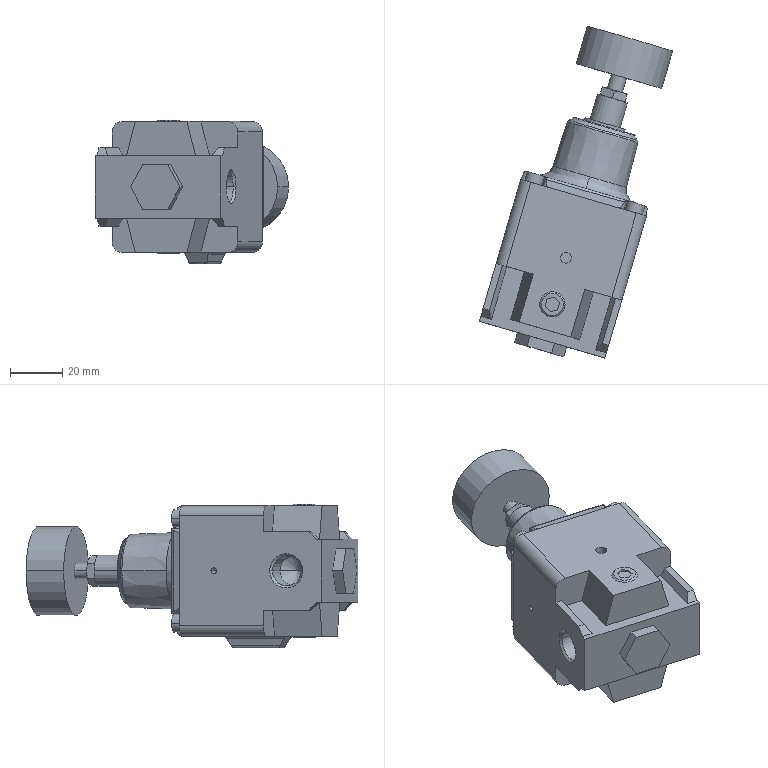Part | SolidWorks | features BaseBody 1 | 1 solid | 182 faces | box 73.887 x 126.864 x 54.9 mm | volume 162557 mm3 | plane 95 | cylinder 53 | cone 28 | spline 6 | commonest cylinder face diameters 2 x11 4 x8 6.8 x8 7.8 x4 8 x4 11.445 x4